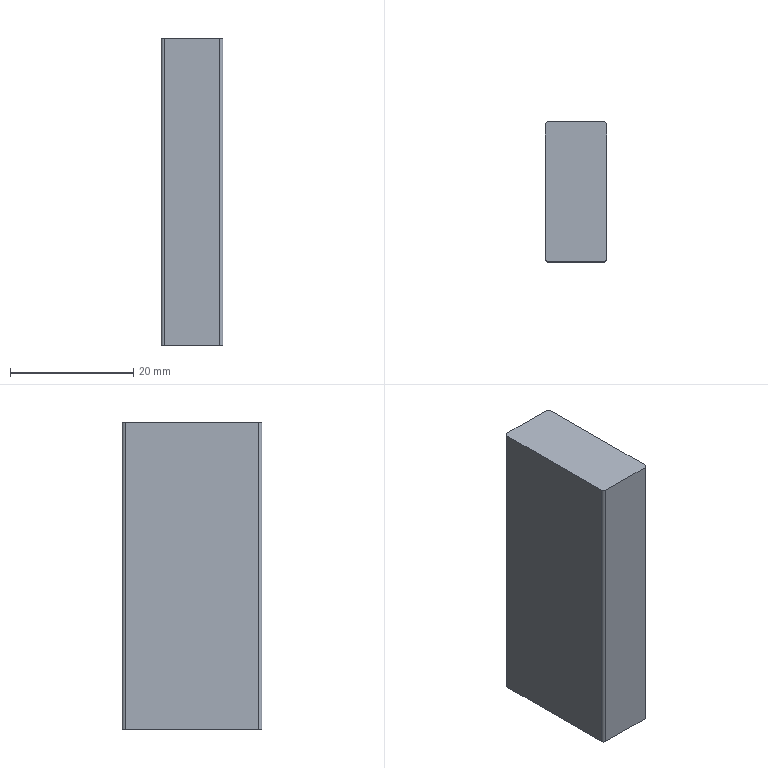Part | NX | features BREP 1 | 1 solid | 10 faces | box 10.05 x 22.702 x 50 mm | volume 11397 mm3 | plane 6 | cylinder 4 | commonest cylinder face diameters 1 x4
STEP:
#1=CARTESIAN_POINT('',(-4.525,11.351,-40.6));
#2=VERTEX_POINT('',#1);
#3=CARTESIAN_POINT('',(-5.025,10.851,-40.6));
#4=VERTEX_POINT('',#3);
#5=CARTESIAN_POINT('',(-4.525,10.851,-40.6));
#6=DIRECTION('',(0.,0.,1.));
#7=DIRECTION('',(1.,0.,0.));
#8=AXIS2_PLACEMENT_3D('',#5,#6,#7);
#9=CIRCLE('',#8,0.5);
#10=EDGE_CURVE('',#2,#4,#9,.T.);
#11=ORIENTED_EDGE('',*,*,#10,.F.);
#12=CARTESIAN_POINT('',(-4.525,11.351,-90.6));
#13=VERTEX_POINT('',#12);
#14=CARTESIAN_POINT('',(-4.525,11.351,-90.6));
#15=DIRECTION('',(0.,0.,1.));
#16=VECTOR('',#15,1000.);
#17=LINE('',#14,#16);
#18=EDGE_CURVE('',#13,#2,#17,.T.);
#19=ORIENTED_EDGE('',*,*,#18,.F.);
#20=CARTESIAN_POINT('',(-5.025,10.851,-90.6));
#21=VERTEX_POINT('',#20);
#22=CARTESIAN_POINT('',(-4.525,10.851,-90.6));
#23=DIRECTION('',(0.,0.,1.));
#24=DIRECTION('',(1.,0.,0.));
#25=AXIS2_PLACEMENT_3D('',#22,#23,#24);
#26=CIRCLE('',#25,0.5);
#27=EDGE_CURVE('',#13,#21,#26,.T.);
#28=ORIENTED_EDGE('',*,*,#27,.T.);
#29=CARTESIAN_POINT('',(-5.025,10.851,-90.6));
#30=DIRECTION('',(0.,0.,1.));
#31=VECTOR('',#30,1000.);
#32=LINE('',#29,#31);
#33=EDGE_CURVE('',#21,#4,#32,.T.);
#34=ORIENTED_EDGE('',*,*,#33,.T.);
#35=EDGE_LOOP('',(#11,#19,#28,#34));
#36=FACE_BOUND('',#35,.T.);
#37=CARTESIAN_POINT('',(-4.525,10.851,-90.6));
#38=DIRECTION('',(0.,0.,1.));
#39=DIRECTION('',(-1.,0.,0.));
#40=AXIS2_PLACEMENT_3D('',#37,#38,#39);
#41=CYLINDRICAL_SURFACE('',#40,0.5);
#42=ADVANCED_FACE('',(#36),#41,.T.);
#43=CARTESIAN_POINT('',(-5.025,-10.851,-40.6));
#44=VERTEX_POINT('',#43);
#45=CARTESIAN_POINT('',(-5.025,-10.851,-40.6));
#46=DIRECTION('',(0.,1.,0.));
#47=VECTOR('',#46,1000.);
#48=LINE('',#45,#47);
#49=EDGE_CURVE('',#44,#4,#48,.T.);
#50=ORIENTED_EDGE('',*,*,#49,.T.);
#51=ORIENTED_EDGE('',*,*,#33,.F.);
#52=CARTESIAN_POINT('',(-5.025,-10.851,-90.6));
#53=VERTEX_POINT('',#52);
#54=CARTESIAN_POINT('',(-5.025,-10.851,-90.6));
#55=DIRECTION('',(0.,1.,0.));
#56=VECTOR('',#55,1000.);
#57=LINE('',#54,#56);
#58=EDGE_CURVE('',#53,#21,#57,.T.);
#59=ORIENTED_EDGE('',*,*,#58,.F.);
#60=CARTESIAN_POINT('',(-5.025,-10.851,-90.6));
#61=DIRECTION('',(0.,0.,1.));
#62=VECTOR('',#61,1000.);
#63=LINE('',#60,#62);
#64=EDGE_CURVE('',#53,#44,#63,.T.);
#65=ORIENTED_EDGE('',*,*,#64,.T.);
#66=EDGE_LOOP('',(#50,#51,#59,#65));
#67=FACE_BOUND('',#66,.T.);
#68=CARTESIAN_POINT('',(-5.025,-10.851,-90.6));
#69=DIRECTION('',(1.,0.,0.));
#70=DIRECTION('',(0.,-1.,0.));
#71=AXIS2_PLACEMENT_3D('',#68,#69,#70);
#72=PLANE('',#71);
#73=ADVANCED_FACE('',(#67),#72,.F.);
#74=CARTESIAN_POINT('',(-4.525,-11.351,-40.6));
#75=VERTEX_POINT('',#74);
#76=CARTESIAN_POINT('',(-4.525,-10.851,-40.6));
#77=DIRECTION('',(0.,0.,1.));
#78=DIRECTION('',(1.,0.,0.));
#79=AXIS2_PLACEMENT_3D('',#76,#77,#78);
#80=CIRCLE('',#79,0.5);
#81=EDGE_CURVE('',#44,#75,#80,.T.);
#82=ORIENTED_EDGE('',*,*,#81,.F.);
#83=ORIENTED_EDGE('',*,*,#64,.F.);
#84=CARTESIAN_POINT('',(-4.525,-11.351,-90.6));
#85=VERTEX_POINT('',#84);
#86=CARTESIAN_POINT('',(-4.525,-10.851,-90.6));
#87=DIRECTION('',(0.,0.,1.));
#88=DIRECTION('',(1.,0.,0.));
#89=AXIS2_PLACEMENT_3D('',#86,#87,#88);
#90=CIRCLE('',#89,0.5);
#91=EDGE_CURVE('',#53,#85,#90,.T.);
#92=ORIENTED_EDGE('',*,*,#91,.T.);
#93=CARTESIAN_POINT('',(-4.525,-11.351,-90.6));
#94=DIRECTION('',(0.,0.,1.));
#95=VECTOR('',#94,1000.);
#96=LINE('',#93,#95);
#97=EDGE_CURVE('',#85,#75,#96,.T.);
#98=ORIENTED_EDGE('',*,*,#97,.T.);
#99=EDGE_LOOP('',(#82,#83,#92,#98));
#100=FACE_BOUND('',#99,.T.);
#101=CARTESIAN_POINT('',(-4.525,-10.851,-90.6));
#102=DIRECTION('',(0.,0.,1.));
#103=DIRECTION('',(-1.,0.,0.));
#104=AXIS2_PLACEMENT_3D('',#101,#102,#103);
#105=CYLINDRICAL_SURFACE('',#104,0.5);
#106=ADVANCED_FACE('',(#100),#105,.T.);
#107=CARTESIAN_POINT('',(4.525,-11.351,-40.6));
#108=VERTEX_POINT('',#107);
#109=CARTESIAN_POINT('',(4.525,-11.351,-40.6));
#110=DIRECTION('',(-1.,0.,0.));
#111=VECTOR('',#110,1000.);
#112=LINE('',#109,#111);
#113=EDGE_CURVE('',#108,#75,#112,.T.);
#114=ORIENTED_EDGE('',*,*,#113,.T.);
#115=ORIENTED_EDGE('',*,*,#97,.F.);
#116=CARTESIAN_POINT('',(4.525,-11.351,-90.6));
#117=VERTEX_POINT('',#116);
#118=CARTESIAN_POINT('',(4.525,-11.351,-90.6));
#119=DIRECTION('',(-1.,0.,0.));
#120=VECTOR('',#119,1000.);
#121=LINE('',#118,#120);
#122=EDGE_CURVE('',#117,#85,#121,.T.);
#123=ORIENTED_EDGE('',*,*,#122,.F.);
#124=CARTESIAN_POINT('',(4.525,-11.351,-90.6));
#125=DIRECTION('',(0.,0.,1.));
#126=VECTOR('',#125,1000.);
#127=LINE('',#124,#126);
#128=EDGE_CURVE('',#117,#108,#127,.T.);
#129=ORIENTED_EDGE('',*,*,#128,.T.);
#130=EDGE_LOOP('',(#114,#115,#123,#129));
#131=FACE_BOUND('',#130,.T.);
#132=CARTESIAN_POINT('',(4.525,-11.351,-90.6));
#133=DIRECTION('',(0.,1.,0.));
#134=DIRECTION('',(1.,0.,0.));
#135=AXIS2_PLACEMENT_3D('',#132,#133,#134);
#136=PLANE('',#135);
#137=ADVANCED_FACE('',(#131),#136,.F.);
#138=CARTESIAN_POINT('',(5.025,-10.851,-40.6));
#139=VERTEX_POINT('',#138);
#140=CARTESIAN_POINT('',(4.525,-10.851,-40.6));
#141=DIRECTION('',(0.,0.,1.));
#142=DIRECTION('',(1.,0.,0.));
#143=AXIS2_PLACEMENT_3D('',#140,#141,#142);
#144=CIRCLE('',#143,0.5);
#145=EDGE_CURVE('',#108,#139,#144,.T.);
#146=ORIENTED_EDGE('',*,*,#145,.F.);
#147=ORIENTED_EDGE('',*,*,#128,.F.);
#148=CARTESIAN_POINT('',(5.025,-10.851,-90.6));
#149=VERTEX_POINT('',#148);
#150=CARTESIAN_POINT('',(4.525,-10.851,-90.6));
#151=DIRECTION('',(0.,0.,1.));
#152=DIRECTION('',(1.,0.,0.));
#153=AXIS2_PLACEMENT_3D('',#150,#151,#152);
#154=CIRCLE('',#153,0.5);
#155=EDGE_CURVE('',#117,#149,#154,.T.);
#156=ORIENTED_EDGE('',*,*,#155,.T.);
#157=CARTESIAN_POINT('',(5.025,-10.851,-90.6));
#158=DIRECTION('',(0.,0.,1.));
#159=VECTOR('',#158,1000.);
#160=LINE('',#157,#159);
#161=EDGE_CURVE('',#149,#139,#160,.T.);
#162=ORIENTED_EDGE('',*,*,#161,.T.);
#163=EDGE_LOOP('',(#146,#147,#156,#162));
#164=FACE_BOUND('',#163,.T.);
#165=CARTESIAN_POINT('',(4.525,-10.851,-90.6));
#166=DIRECTION('',(0.,0.,1.));
#167=DIRECTION('',(-1.,0.,0.));
#168=AXIS2_PLACEMENT_3D('',#165,#166,#167);
#169=CYLINDRICAL_SURFACE('',#168,0.5);
#170=ADVANCED_FACE('',(#164),#169,.T.);
#171=CARTESIAN_POINT('',(5.025,10.851,-40.6));
#172=VERTEX_POINT('',#171);
#173=CARTESIAN_POINT('',(5.025,10.851,-40.6));
#174=DIRECTION('',(0.,-1.,0.));
#175=VECTOR('',#174,1000.);
#176=LINE('',#173,#175);
#177=EDGE_CURVE('',#172,#139,#176,.T.);
#178=ORIENTED_EDGE('',*,*,#177,.T.);
#179=ORIENTED_EDGE('',*,*,#161,.F.);
#180=CARTESIAN_POINT('',(5.025,10.851,-90.6));
#181=VERTEX_POINT('',#180);
#182=CARTESIAN_POINT('',(5.025,10.851,-90.6));
#183=DIRECTION('',(0.,-1.,0.));
#184=VECTOR('',#183,1000.);
#185=LINE('',#182,#184);
#186=EDGE_CURVE('',#181,#149,#185,.T.);
#187=ORIENTED_EDGE('',*,*,#186,.F.);
#188=CARTESIAN_POINT('',(5.025,10.851,-90.6));
#189=DIRECTION('',(0.,0.,1.));
#190=VECTOR('',#189,1000.);
#191=LINE('',#188,#190);
#192=EDGE_CURVE('',#181,#172,#191,.T.);
#193=ORIENTED_EDGE('',*,*,#192,.T.);
#194=EDGE_LOOP('',(#178,#179,#187,#193));
#195=FACE_BOUND('',#194,.T.);
#196=CARTESIAN_POINT('',(5.025,10.851,-90.6));
#197=DIRECTION('',(-1.,0.,0.));
#198=DIRECTION('',(0.,0.,-1.));
#199=AXIS2_PLACEMENT_3D('',#196,#197,#198);
#200=PLANE('',#199);
#201=ADVANCED_FACE('',(#195),#200,.F.);
#202=CARTESIAN_POINT('',(4.525,11.351,-40.6));
#203=VERTEX_POINT('',#202);
#204=CARTESIAN_POINT('',(4.525,10.851,-40.6));
#205=DIRECTION('',(0.,0.,1.));
#206=DIRECTION('',(1.,0.,0.));
#207=AXIS2_PLACEMENT_3D('',#204,#205,#206);
#208=CIRCLE('',#207,0.5);
#209=EDGE_CURVE('',#172,#203,#208,.T.);
#210=ORIENTED_EDGE('',*,*,#209,.F.);
#211=ORIENTED_EDGE('',*,*,#192,.F.);
#212=CARTESIAN_POINT('',(4.525,11.351,-90.6));
#213=VERTEX_POINT('',#212);
#214=CARTESIAN_POINT('',(4.525,10.851,-90.6));
#215=DIRECTION('',(0.,0.,1.));
#216=DIRECTION('',(1.,0.,0.));
#217=AXIS2_PLACEMENT_3D('',#214,#215,#216);
#218=CIRCLE('',#217,0.5);
#219=EDGE_CURVE('',#181,#213,#218,.T.);
#220=ORIENTED_EDGE('',*,*,#219,.T.);
#221=CARTESIAN_POINT('',(4.525,11.351,-90.6));
#222=DIRECTION('',(0.,0.,1.));
#223=VECTOR('',#222,1000.);
#224=LINE('',#221,#223);
#225=EDGE_CURVE('',#213,#203,#224,.T.);
#226=ORIENTED_EDGE('',*,*,#225,.T.);
#227=EDGE_LOOP('',(#210,#211,#220,#226));
#228=FACE_BOUND('',#227,.T.);
#229=CARTESIAN_POINT('',(4.525,10.851,-90.6));
#230=DIRECTION('',(0.,0.,1.));
#231=DIRECTION('',(-1.,0.,0.));
#232=AXIS2_PLACEMENT_3D('',#229,#230,#231);
#233=CYLINDRICAL_SURFACE('',#232,0.5);
#234=ADVANCED_FACE('',(#228),#233,.T.);
#235=CARTESIAN_POINT('',(-4.525,11.351,-40.6));
#236=DIRECTION('',(1.,0.,0.));
#237=VECTOR('',#236,1000.);
#238=LINE('',#235,#237);
#239=EDGE_CURVE('',#2,#203,#238,.T.);
#240=ORIENTED_EDGE('',*,*,#239,.T.);
#241=ORIENTED_EDGE('',*,*,#225,.F.);
#242=CARTESIAN_POINT('',(-4.525,11.351,-90.6));
#243=DIRECTION('',(1.,0.,0.));
#244=VECTOR('',#243,1000.);
#245=LINE('',#242,#244);
#246=EDGE_CURVE('',#13,#213,#245,.T.);
#247=ORIENTED_EDGE('',*,*,#246,.F.);
#248=ORIENTED_EDGE('',*,*,#18,.T.);
#249=EDGE_LOOP('',(#240,#241,#247,#248));
#250=FACE_BOUND('',#249,.T.);
#251=CARTESIAN_POINT('',(-4.525,11.351,-90.6));
#252=DIRECTION('',(0.,-1.,0.));
#253=DIRECTION('',(-1.,0.,0.));
#254=AXIS2_PLACEMENT_3D('',#251,#252,#253);
#255=PLANE('',#254);
#256=ADVANCED_FACE('',(#250),#255,.F.);
#257=ORIENTED_EDGE('',*,*,#27,.F.);
#258=ORIENTED_EDGE('',*,*,#246,.T.);
#259=ORIENTED_EDGE('',*,*,#219,.F.);
#260=ORIENTED_EDGE('',*,*,#186,.T.);
#261=ORIENTED_EDGE('',*,*,#155,.F.);
#262=ORIENTED_EDGE('',*,*,#122,.T.);
#263=ORIENTED_EDGE('',*,*,#91,.F.);
#264=ORIENTED_EDGE('',*,*,#58,.T.);
#265=EDGE_LOOP('',(#257,#258,#259,#260,#261,#262,#263,#264));
#266=FACE_BOUND('',#265,.T.);
#267=CARTESIAN_POINT('',(-4.525,10.851,-90.6));
#268=DIRECTION('',(0.,0.,1.));
#269=DIRECTION('',(-1.,0.,0.));
#270=AXIS2_PLACEMENT_3D('',#267,#268,#269);
#271=PLANE('',#270);
#272=ADVANCED_FACE('',(#266),#271,.F.);
#273=ORIENTED_EDGE('',*,*,#10,.T.);
#274=ORIENTED_EDGE('',*,*,#49,.F.);
#275=ORIENTED_EDGE('',*,*,#81,.T.);
#276=ORIENTED_EDGE('',*,*,#113,.F.);
#277=ORIENTED_EDGE('',*,*,#145,.T.);
#278=ORIENTED_EDGE('',*,*,#177,.F.);
#279=ORIENTED_EDGE('',*,*,#209,.T.);
#280=ORIENTED_EDGE('',*,*,#239,.F.);
#281=EDGE_LOOP('',(#273,#274,#275,#276,#277,#278,#279,#280));
#282=FACE_BOUND('',#281,.T.);
#283=CARTESIAN_POINT('',(-4.525,10.851,-40.6));
#284=DIRECTION('',(0.,0.,1.));
#285=DIRECTION('',(-1.,0.,0.));
#286=AXIS2_PLACEMENT_3D('',#283,#284,#285);
#287=PLANE('',#286);
#288=ADVANCED_FACE('',(#282),#287,.T.);
#289=CLOSED_SHELL('',(#42,#73,#106,#137,#170,#201,#234,#256,#272,#288));
#290=MANIFOLD_SOLID_BREP('',#289);
#291=(LENGTH_UNIT()NAMED_UNIT(*)SI_UNIT(.MILLI.,.METRE.));
#292=UNCERTAINTY_MEASURE_WITH_UNIT(LENGTH_MEASURE(0.00001),#291,'','');
#293=(NAMED_UNIT(*)PLANE_ANGLE_UNIT()SI_UNIT($,.RADIAN.));
#294=(NAMED_UNIT(*)SI_UNIT($,.STERADIAN.)SOLID_ANGLE_UNIT());
#295=(GEOMETRIC_REPRESENTATION_CONTEXT(3)GLOBAL_UNCERTAINTY_ASSIGNED_CONTEXT((#292))GLOBAL_UNIT_ASSIGNED_CONTEXT((#291,#293,#294))REPRESENTATION_CONTEXT('',''));
#296=ADVANCED_BREP_SHAPE_REPRESENTATION('',(#290),#295);